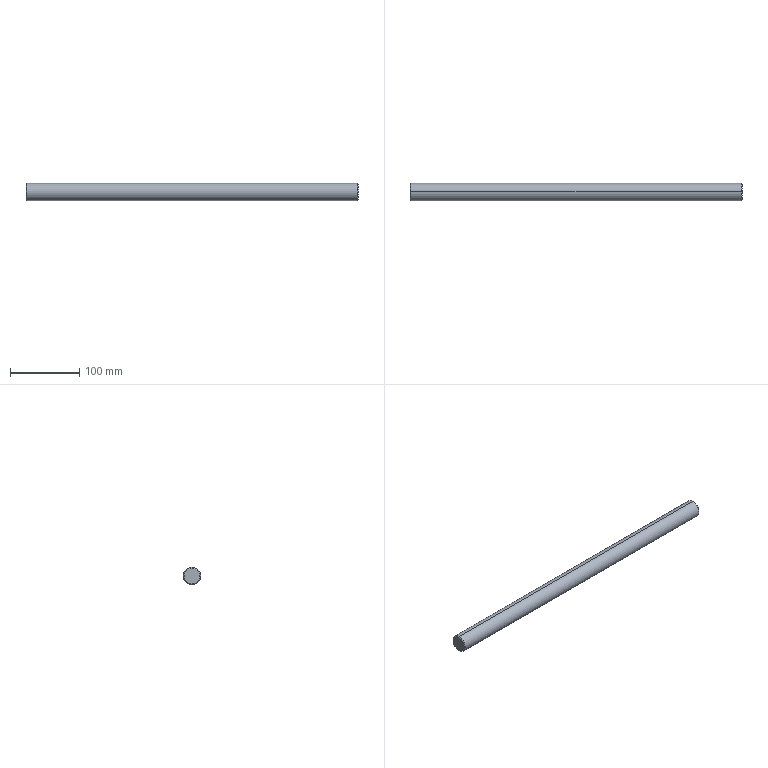Part | SolidWorks | features Chamfer 1, Extrusion 1 | 1 solid | 8 faces | box 480 x 25 x 25 mm | volume 235543 mm3 | cone 4 | cylinder 2 | plane 2 | commonest cylinder face diameters 25 x2
STEP:
#1=CARTESIAN_POINT('',(0.,0.,11.5));
#2=VERTEX_POINT('',#1);
#3=CARTESIAN_POINT('',(0.,0.,-11.5));
#4=VERTEX_POINT('',#3);
#5=CARTESIAN_POINT('',(0.,0.,0.));
#6=DIRECTION('',(-1.,0.,0.));
#7=DIRECTION('',(0.,0.,-1.));
#8=AXIS2_PLACEMENT_3D('',#5,#6,#7);
#9=CIRCLE('',#8,11.5);
#10=EDGE_CURVE('',#2,#4,#9,.T.);
#11=ORIENTED_EDGE('',*,*,#10,.F.);
#12=CARTESIAN_POINT('',(1.,0.,12.5));
#13=VERTEX_POINT('',#12);
#14=CARTESIAN_POINT('',(1.,0.,12.5));
#15=DIRECTION('',(0.7071,0.,0.7071));
#16=VECTOR('',#15,1000.);
#17=LINE('',#14,#16);
#18=EDGE_CURVE('',#2,#13,#17,.T.);
#19=ORIENTED_EDGE('',*,*,#18,.T.);
#20=CARTESIAN_POINT('',(1.,0.,-12.5));
#21=VERTEX_POINT('',#20);
#22=CARTESIAN_POINT('',(1.,0.,0.));
#23=DIRECTION('',(1.,0.,0.));
#24=DIRECTION('',(0.,0.,-1.));
#25=AXIS2_PLACEMENT_3D('',#22,#23,#24);
#26=CIRCLE('',#25,12.5);
#27=EDGE_CURVE('',#21,#13,#26,.T.);
#28=ORIENTED_EDGE('',*,*,#27,.F.);
#29=CARTESIAN_POINT('',(1.,0.,-12.5));
#30=DIRECTION('',(0.7071,0.,-0.7071));
#31=VECTOR('',#30,1000.);
#32=LINE('',#29,#31);
#33=EDGE_CURVE('',#4,#21,#32,.T.);
#34=ORIENTED_EDGE('',*,*,#33,.F.);
#35=EDGE_LOOP('',(#11,#19,#28,#34));
#36=FACE_OUTER_BOUND('',#35,.T.);
#37=CARTESIAN_POINT('',(1.,0.,0.));
#38=DIRECTION('',(1.,0.,0.));
#39=DIRECTION('',(0.,0.,-1.));
#40=AXIS2_PLACEMENT_3D('',#37,#38,#39);
#41=CONICAL_SURFACE('',#40,12.5,0.7854);
#42=ADVANCED_FACE('',(#36),#41,.T.);
#43=CARTESIAN_POINT('',(480.,0.,-11.5));
#44=VERTEX_POINT('',#43);
#45=CARTESIAN_POINT('',(480.,0.,11.5));
#46=VERTEX_POINT('',#45);
#47=CARTESIAN_POINT('',(480.,0.,0.));
#48=DIRECTION('',(1.,0.,0.));
#49=DIRECTION('',(0.,0.,-1.));
#50=AXIS2_PLACEMENT_3D('',#47,#48,#49);
#51=CIRCLE('',#50,11.5);
#52=EDGE_CURVE('',#44,#46,#51,.T.);
#53=ORIENTED_EDGE('',*,*,#52,.F.);
#54=CARTESIAN_POINT('',(479.,0.,-12.5));
#55=VERTEX_POINT('',#54);
#56=CARTESIAN_POINT('',(480.,0.,-11.5));
#57=DIRECTION('',(-0.7071,0.,-0.7071));
#58=VECTOR('',#57,1000.);
#59=LINE('',#56,#58);
#60=EDGE_CURVE('',#44,#55,#59,.T.);
#61=ORIENTED_EDGE('',*,*,#60,.T.);
#62=CARTESIAN_POINT('',(479.,0.,12.5));
#63=VERTEX_POINT('',#62);
#64=CARTESIAN_POINT('',(479.,0.,0.));
#65=DIRECTION('',(-1.,0.,0.));
#66=DIRECTION('',(0.,0.,-1.));
#67=AXIS2_PLACEMENT_3D('',#64,#65,#66);
#68=CIRCLE('',#67,12.5);
#69=EDGE_CURVE('',#63,#55,#68,.T.);
#70=ORIENTED_EDGE('',*,*,#69,.F.);
#71=CARTESIAN_POINT('',(480.,0.,11.5));
#72=DIRECTION('',(-0.7071,0.,0.7071));
#73=VECTOR('',#72,1000.);
#74=LINE('',#71,#73);
#75=EDGE_CURVE('',#46,#63,#74,.T.);
#76=ORIENTED_EDGE('',*,*,#75,.F.);
#77=EDGE_LOOP('',(#53,#61,#70,#76));
#78=FACE_OUTER_BOUND('',#77,.T.);
#79=CARTESIAN_POINT('',(480.,0.,0.));
#80=DIRECTION('',(-1.,0.,0.));
#81=DIRECTION('',(0.,0.,1.));
#82=AXIS2_PLACEMENT_3D('',#79,#80,#81);
#83=CONICAL_SURFACE('',#82,11.5,0.7854);
#84=ADVANCED_FACE('',(#78),#83,.T.);
#85=ORIENTED_EDGE('',*,*,#69,.T.);
#86=CARTESIAN_POINT('',(480.,0.,-12.5));
#87=DIRECTION('',(-1.,0.,0.));
#88=VECTOR('',#87,1000.);
#89=LINE('',#86,#88);
#90=EDGE_CURVE('',#55,#21,#89,.T.);
#91=ORIENTED_EDGE('',*,*,#90,.T.);
#92=ORIENTED_EDGE('',*,*,#27,.T.);
#93=CARTESIAN_POINT('',(480.,0.,12.5));
#94=DIRECTION('',(-1.,0.,0.));
#95=VECTOR('',#94,1000.);
#96=LINE('',#93,#95);
#97=EDGE_CURVE('',#63,#13,#96,.T.);
#98=ORIENTED_EDGE('',*,*,#97,.F.);
#99=EDGE_LOOP('',(#85,#91,#92,#98));
#100=FACE_OUTER_BOUND('',#99,.T.);
#101=CARTESIAN_POINT('',(480.,0.,0.));
#102=DIRECTION('',(-1.,0.,0.));
#103=DIRECTION('',(0.,0.,1.));
#104=AXIS2_PLACEMENT_3D('',#101,#102,#103);
#105=CYLINDRICAL_SURFACE('',#104,12.5);
#106=ADVANCED_FACE('',(#100),#105,.T.);
#107=ORIENTED_EDGE('',*,*,#90,.F.);
#108=CARTESIAN_POINT('',(479.,0.,0.));
#109=DIRECTION('',(-1.,0.,0.));
#110=DIRECTION('',(0.,0.,-1.));
#111=AXIS2_PLACEMENT_3D('',#108,#109,#110);
#112=CIRCLE('',#111,12.5);
#113=EDGE_CURVE('',#55,#63,#112,.T.);
#114=ORIENTED_EDGE('',*,*,#113,.T.);
#115=ORIENTED_EDGE('',*,*,#97,.T.);
#116=CARTESIAN_POINT('',(1.,0.,0.));
#117=DIRECTION('',(1.,0.,0.));
#118=DIRECTION('',(0.,0.,-1.));
#119=AXIS2_PLACEMENT_3D('',#116,#117,#118);
#120=CIRCLE('',#119,12.5);
#121=EDGE_CURVE('',#13,#21,#120,.T.);
#122=ORIENTED_EDGE('',*,*,#121,.T.);
#123=EDGE_LOOP('',(#107,#114,#115,#122));
#124=FACE_OUTER_BOUND('',#123,.T.);
#125=CARTESIAN_POINT('',(480.,0.,0.));
#126=DIRECTION('',(-1.,0.,0.));
#127=DIRECTION('',(0.,0.,1.));
#128=AXIS2_PLACEMENT_3D('',#125,#126,#127);
#129=CYLINDRICAL_SURFACE('',#128,12.5);
#130=ADVANCED_FACE('',(#124),#129,.T.);
#131=CARTESIAN_POINT('',(480.,0.,0.));
#132=DIRECTION('',(1.,0.,0.));
#133=DIRECTION('',(0.,0.,-1.));
#134=AXIS2_PLACEMENT_3D('',#131,#132,#133);
#135=CIRCLE('',#134,11.5);
#136=EDGE_CURVE('',#46,#44,#135,.T.);
#137=ORIENTED_EDGE('',*,*,#136,.T.);
#138=ORIENTED_EDGE('',*,*,#52,.T.);
#139=EDGE_LOOP('',(#137,#138));
#140=FACE_OUTER_BOUND('',#139,.T.);
#141=CARTESIAN_POINT('',(480.,0.,0.));
#142=DIRECTION('',(1.,0.,0.));
#143=DIRECTION('',(0.,0.,-1.));
#144=AXIS2_PLACEMENT_3D('',#141,#142,#143);
#145=PLANE('',#144);
#146=ADVANCED_FACE('',(#140),#145,.T.);
#147=CARTESIAN_POINT('',(0.,0.,0.));
#148=DIRECTION('',(-1.,0.,0.));
#149=DIRECTION('',(0.,0.,-1.));
#150=AXIS2_PLACEMENT_3D('',#147,#148,#149);
#151=CIRCLE('',#150,11.5);
#152=EDGE_CURVE('',#4,#2,#151,.T.);
#153=ORIENTED_EDGE('',*,*,#152,.T.);
#154=ORIENTED_EDGE('',*,*,#10,.T.);
#155=EDGE_LOOP('',(#153,#154));
#156=FACE_OUTER_BOUND('',#155,.T.);
#157=CARTESIAN_POINT('',(0.,0.,0.));
#158=DIRECTION('',(1.,0.,0.));
#159=DIRECTION('',(0.,0.,-1.));
#160=AXIS2_PLACEMENT_3D('',#157,#158,#159);
#161=PLANE('',#160);
#162=ADVANCED_FACE('',(#156),#161,.F.);
#163=ORIENTED_EDGE('',*,*,#60,.F.);
#164=ORIENTED_EDGE('',*,*,#136,.F.);
#165=ORIENTED_EDGE('',*,*,#75,.T.);
#166=ORIENTED_EDGE('',*,*,#113,.F.);
#167=EDGE_LOOP('',(#163,#164,#165,#166));
#168=FACE_OUTER_BOUND('',#167,.T.);
#169=CARTESIAN_POINT('',(480.,0.,0.));
#170=DIRECTION('',(-1.,0.,0.));
#171=DIRECTION('',(0.,0.,1.));
#172=AXIS2_PLACEMENT_3D('',#169,#170,#171);
#173=CONICAL_SURFACE('',#172,11.5,0.7854);
#174=ADVANCED_FACE('',(#168),#173,.T.);
#175=ORIENTED_EDGE('',*,*,#18,.F.);
#176=ORIENTED_EDGE('',*,*,#152,.F.);
#177=ORIENTED_EDGE('',*,*,#33,.T.);
#178=ORIENTED_EDGE('',*,*,#121,.F.);
#179=EDGE_LOOP('',(#175,#176,#177,#178));
#180=FACE_OUTER_BOUND('',#179,.T.);
#181=CARTESIAN_POINT('',(1.,0.,0.));
#182=DIRECTION('',(1.,0.,0.));
#183=DIRECTION('',(0.,0.,-1.));
#184=AXIS2_PLACEMENT_3D('',#181,#182,#183);
#185=CONICAL_SURFACE('',#184,12.5,0.7854);
#186=ADVANCED_FACE('',(#180),#185,.T.);
#187=CLOSED_SHELL('',(#42,#84,#106,#130,#146,#162,#174,#186));
#188=MANIFOLD_SOLID_BREP('',#187);
#189=CARTESIAN_POINT('',(0.,0.,0.));
#190=DIRECTION('',(0.,0.,1.));
#191=DIRECTION('',(1.,0.,0.));
#192=AXIS2_PLACEMENT_3D('',#189,#190,#191);
#193=(LENGTH_UNIT()NAMED_UNIT(*)SI_UNIT(.MILLI.,.METRE.));
#194=UNCERTAINTY_MEASURE_WITH_UNIT(LENGTH_MEASURE(0.00001),#193,'','');
#195=(NAMED_UNIT(*)PLANE_ANGLE_UNIT()SI_UNIT($,.RADIAN.));
#196=(NAMED_UNIT(*)SI_UNIT($,.STERADIAN.)SOLID_ANGLE_UNIT());
#197=(GEOMETRIC_REPRESENTATION_CONTEXT(3)GLOBAL_UNCERTAINTY_ASSIGNED_CONTEXT((#194))GLOBAL_UNIT_ASSIGNED_CONTEXT((#193,#195,#196))REPRESENTATION_CONTEXT('',''));
#198=ADVANCED_BREP_SHAPE_REPRESENTATION('',(#188,#192),#197);